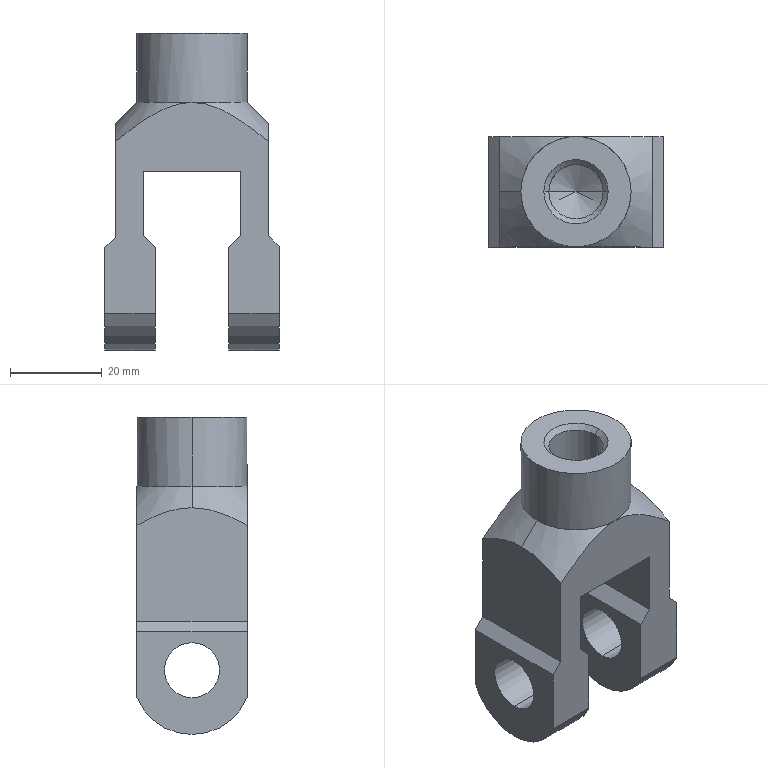Part | STEP file | Y_040B_Y-040B | 1 solid | 35 faces | box 38 x 24 x 69 mm | volume 28298 mm3 | plane 16 | cylinder 12 | cone 7 | commonest cylinder face diameters 12 x4 26 x4 11.84 x2 24 x2
STEP:
#1=CARTESIAN_POINT('',(0.,0.,-26.418));
#2=VERTEX_POINT('',#1);
#3=CARTESIAN_POINT('',(5.92,0.,-23.));
#4=VERTEX_POINT('',#3);
#5=CARTESIAN_POINT('',(0.,0.,-26.418));
#6=DIRECTION('',(0.866,0.,0.5));
#7=VECTOR('',#6,1000.);
#8=LINE('',#5,#7);
#9=EDGE_CURVE('',#2,#4,#8,.T.);
#10=ORIENTED_EDGE('',*,*,#9,.F.);
#11=CARTESIAN_POINT('',(-5.92,0.,-23.));
#12=VERTEX_POINT('',#11);
#13=CARTESIAN_POINT('',(0.,0.,-26.418));
#14=DIRECTION('',(-0.866,0.,0.5));
#15=VECTOR('',#14,1000.);
#16=LINE('',#13,#15);
#17=EDGE_CURVE('',#2,#12,#16,.T.);
#18=ORIENTED_EDGE('',*,*,#17,.T.);
#19=CARTESIAN_POINT('',(0.,0.,-23.));
#20=DIRECTION('',(0.,0.,1.));
#21=DIRECTION('',(1.,0.,0.));
#22=AXIS2_PLACEMENT_3D('',#19,#20,#21);
#23=CIRCLE('',#22,5.92);
#24=EDGE_CURVE('',#12,#4,#23,.T.);
#25=ORIENTED_EDGE('',*,*,#24,.T.);
#26=EDGE_LOOP('',(#10,#18,#25));
#27=FACE_OUTER_BOUND('',#26,.T.);
#28=CARTESIAN_POINT('',(0.,0.,973.582));
#29=DIRECTION('',(0.,0.,1.));
#30=DIRECTION('',(1.,0.,0.));
#31=AXIS2_PLACEMENT_3D('',#28,#29,#30);
#32=CONICAL_SURFACE('',#31,1732.051,1.047);
#33=ADVANCED_FACE('',(#27),#32,.F.);
#34=ORIENTED_EDGE('',*,*,#24,.F.);
#35=CARTESIAN_POINT('',(-5.92,0.,-1.08));
#36=VERTEX_POINT('',#35);
#37=CARTESIAN_POINT('',(-5.92,0.,-26.418));
#38=DIRECTION('',(0.,0.,1.));
#39=VECTOR('',#38,1000.);
#40=LINE('',#37,#39);
#41=EDGE_CURVE('',#12,#36,#40,.T.);
#42=ORIENTED_EDGE('',*,*,#41,.T.);
#43=CARTESIAN_POINT('',(5.92,0.,-1.08));
#44=VERTEX_POINT('',#43);
#45=CARTESIAN_POINT('',(0.,0.,-1.08));
#46=DIRECTION('',(0.,0.,1.));
#47=DIRECTION('',(1.,0.,0.));
#48=AXIS2_PLACEMENT_3D('',#45,#46,#47);
#49=CIRCLE('',#48,5.92);
#50=EDGE_CURVE('',#36,#44,#49,.T.);
#51=ORIENTED_EDGE('',*,*,#50,.T.);
#52=CARTESIAN_POINT('',(5.92,0.,-26.418));
#53=DIRECTION('',(0.,0.,1.));
#54=VECTOR('',#53,1000.);
#55=LINE('',#52,#54);
#56=EDGE_CURVE('',#4,#44,#55,.T.);
#57=ORIENTED_EDGE('',*,*,#56,.F.);
#58=EDGE_LOOP('',(#34,#42,#51,#57));
#59=FACE_OUTER_BOUND('',#58,.T.);
#60=CARTESIAN_POINT('',(0.,0.,-26.418));
#61=DIRECTION('',(0.,0.,1.));
#62=DIRECTION('',(1.,0.,0.));
#63=AXIS2_PLACEMENT_3D('',#60,#61,#62);
#64=CYLINDRICAL_SURFACE('',#63,5.92);
#65=ADVANCED_FACE('',(#59),#64,.F.);
#66=ORIENTED_EDGE('',*,*,#50,.F.);
#67=CARTESIAN_POINT('',(-7.,0.,0.));
#68=VERTEX_POINT('',#67);
#69=CARTESIAN_POINT('',(-5.92,0.,-1.08));
#70=DIRECTION('',(-0.7071,0.,0.7071));
#71=VECTOR('',#70,1000.);
#72=LINE('',#69,#71);
#73=EDGE_CURVE('',#36,#68,#72,.T.);
#74=ORIENTED_EDGE('',*,*,#73,.T.);
#75=CARTESIAN_POINT('',(7.,0.,0.));
#76=VERTEX_POINT('',#75);
#77=CARTESIAN_POINT('',(0.,0.,0.));
#78=DIRECTION('',(0.,0.,1.));
#79=DIRECTION('',(-1.,0.,0.));
#80=AXIS2_PLACEMENT_3D('',#77,#78,#79);
#81=CIRCLE('',#80,7.);
#82=EDGE_CURVE('',#68,#76,#81,.T.);
#83=ORIENTED_EDGE('',*,*,#82,.T.);
#84=CARTESIAN_POINT('',(5.92,0.,-1.08));
#85=DIRECTION('',(0.7071,0.,0.7071));
#86=VECTOR('',#85,1000.);
#87=LINE('',#84,#86);
#88=EDGE_CURVE('',#44,#76,#87,.T.);
#89=ORIENTED_EDGE('',*,*,#88,.F.);
#90=EDGE_LOOP('',(#66,#74,#83,#89));
#91=FACE_OUTER_BOUND('',#90,.T.);
#92=CARTESIAN_POINT('',(0.,0.,-1.08));
#93=DIRECTION('',(0.,0.,1.));
#94=DIRECTION('',(1.,0.,0.));
#95=AXIS2_PLACEMENT_3D('',#92,#93,#94);
#96=CONICAL_SURFACE('',#95,5.92,0.7854);
#97=ADVANCED_FACE('',(#91),#96,.F.);
#98=CARTESIAN_POINT('',(8.,0.,-49.));
#99=VERTEX_POINT('',#98);
#100=CARTESIAN_POINT('',(8.,0.,-61.));
#101=VERTEX_POINT('',#100);
#102=CARTESIAN_POINT('',(8.,0.,-55.));
#103=DIRECTION('',(1.,0.,0.));
#104=DIRECTION('',(0.,0.,-1.));
#105=AXIS2_PLACEMENT_3D('',#102,#103,#104);
#106=CIRCLE('',#105,6.);
#107=EDGE_CURVE('',#99,#101,#106,.T.);
#108=ORIENTED_EDGE('',*,*,#107,.F.);
#109=CARTESIAN_POINT('',(19.,0.,-49.));
#110=VERTEX_POINT('',#109);
#111=CARTESIAN_POINT('',(-24.,0.,-49.));
#112=DIRECTION('',(1.,0.,0.));
#113=VECTOR('',#112,1000.);
#114=LINE('',#111,#113);
#115=EDGE_CURVE('',#99,#110,#114,.T.);
#116=ORIENTED_EDGE('',*,*,#115,.T.);
#117=CARTESIAN_POINT('',(19.,0.,-61.));
#118=VERTEX_POINT('',#117);
#119=CARTESIAN_POINT('',(19.,0.,-55.));
#120=DIRECTION('',(-1.,0.,0.));
#121=DIRECTION('',(0.,0.,1.));
#122=AXIS2_PLACEMENT_3D('',#119,#120,#121);
#123=CIRCLE('',#122,6.);
#124=EDGE_CURVE('',#118,#110,#123,.T.);
#125=ORIENTED_EDGE('',*,*,#124,.F.);
#126=CARTESIAN_POINT('',(-24.,0.,-61.));
#127=DIRECTION('',(1.,0.,0.));
#128=VECTOR('',#127,1000.);
#129=LINE('',#126,#128);
#130=EDGE_CURVE('',#101,#118,#129,.T.);
#131=ORIENTED_EDGE('',*,*,#130,.F.);
#132=EDGE_LOOP('',(#108,#116,#125,#131));
#133=FACE_OUTER_BOUND('',#132,.T.);
#134=CARTESIAN_POINT('',(-24.,0.,-55.));
#135=DIRECTION('',(1.,0.,0.));
#136=DIRECTION('',(0.,0.,-1.));
#137=AXIS2_PLACEMENT_3D('',#134,#135,#136);
#138=CYLINDRICAL_SURFACE('',#137,6.);
#139=ADVANCED_FACE('',(#133),#138,.F.);
#140=CARTESIAN_POINT('',(-19.,0.,-49.));
#141=VERTEX_POINT('',#140);
#142=CARTESIAN_POINT('',(-19.,0.,-61.));
#143=VERTEX_POINT('',#142);
#144=CARTESIAN_POINT('',(-19.,0.,-55.));
#145=DIRECTION('',(1.,0.,0.));
#146=DIRECTION('',(0.,0.,-1.));
#147=AXIS2_PLACEMENT_3D('',#144,#145,#146);
#148=CIRCLE('',#147,6.);
#149=EDGE_CURVE('',#141,#143,#148,.T.);
#150=ORIENTED_EDGE('',*,*,#149,.F.);
#151=CARTESIAN_POINT('',(-8.,0.,-49.));
#152=VERTEX_POINT('',#151);
#153=CARTESIAN_POINT('',(-24.,0.,-49.));
#154=DIRECTION('',(1.,0.,0.));
#155=VECTOR('',#154,1000.);
#156=LINE('',#153,#155);
#157=EDGE_CURVE('',#141,#152,#156,.T.);
#158=ORIENTED_EDGE('',*,*,#157,.T.);
#159=CARTESIAN_POINT('',(-8.,0.,-61.));
#160=VERTEX_POINT('',#159);
#161=CARTESIAN_POINT('',(-8.,0.,-55.));
#162=DIRECTION('',(-1.,0.,0.));
#163=DIRECTION('',(0.,0.,1.));
#164=AXIS2_PLACEMENT_3D('',#161,#162,#163);
#165=CIRCLE('',#164,6.);
#166=EDGE_CURVE('',#160,#152,#165,.T.);
#167=ORIENTED_EDGE('',*,*,#166,.F.);
#168=CARTESIAN_POINT('',(-24.,0.,-61.));
#169=DIRECTION('',(1.,0.,0.));
#170=VECTOR('',#169,1000.);
#171=LINE('',#168,#170);
#172=EDGE_CURVE('',#143,#160,#171,.T.);
#173=ORIENTED_EDGE('',*,*,#172,.F.);
#174=EDGE_LOOP('',(#150,#158,#167,#173));
#175=FACE_OUTER_BOUND('',#174,.T.);
#176=CARTESIAN_POINT('',(-24.,0.,-55.));
#177=DIRECTION('',(1.,0.,0.));
#178=DIRECTION('',(0.,0.,-1.));
#179=AXIS2_PLACEMENT_3D('',#176,#177,#178);
#180=CYLINDRICAL_SURFACE('',#179,6.);
#181=ADVANCED_FACE('',(#175),#180,.F.);
#182=CARTESIAN_POINT('',(8.,0.,-69.));
#183=VERTEX_POINT('',#182);
#184=CARTESIAN_POINT('',(8.,-12.,-61.));
#185=VERTEX_POINT('',#184);
#186=CARTESIAN_POINT('',(8.,0.,-56.));
#187=DIRECTION('',(-1.,0.,0.));
#188=DIRECTION('',(0.,0.,-1.));
#189=AXIS2_PLACEMENT_3D('',#186,#187,#188);
#190=CIRCLE('',#189,13.);
#191=EDGE_CURVE('',#183,#185,#190,.T.);
#192=ORIENTED_EDGE('',*,*,#191,.F.);
#193=CARTESIAN_POINT('',(19.,0.,-69.));
#194=VERTEX_POINT('',#193);
#195=CARTESIAN_POINT('',(-24.,0.,-69.));
#196=DIRECTION('',(1.,0.,0.));
#197=VECTOR('',#196,1000.);
#198=LINE('',#195,#197);
#199=EDGE_CURVE('',#183,#194,#198,.T.);
#200=ORIENTED_EDGE('',*,*,#199,.T.);
#201=CARTESIAN_POINT('',(19.,-12.,-61.));
#202=VERTEX_POINT('',#201);
#203=CARTESIAN_POINT('',(19.,0.,-56.));
#204=DIRECTION('',(1.,0.,0.));
#205=DIRECTION('',(0.,0.,1.));
#206=AXIS2_PLACEMENT_3D('',#203,#204,#205);
#207=CIRCLE('',#206,13.);
#208=EDGE_CURVE('',#202,#194,#207,.T.);
#209=ORIENTED_EDGE('',*,*,#208,.F.);
#210=CARTESIAN_POINT('',(-24.,-12.,-61.));
#211=DIRECTION('',(1.,0.,0.));
#212=VECTOR('',#211,1000.);
#213=LINE('',#210,#212);
#214=EDGE_CURVE('',#185,#202,#213,.T.);
#215=ORIENTED_EDGE('',*,*,#214,.F.);
#216=EDGE_LOOP('',(#192,#200,#209,#215));
#217=FACE_OUTER_BOUND('',#216,.T.);
#218=CARTESIAN_POINT('',(-24.,0.,-56.));
#219=DIRECTION('',(1.,0.,0.));
#220=DIRECTION('',(0.,0.,-1.));
#221=AXIS2_PLACEMENT_3D('',#218,#219,#220);
#222=CYLINDRICAL_SURFACE('',#221,13.);
#223=ADVANCED_FACE('',(#217),#222,.T.);
#224=CARTESIAN_POINT('',(-19.,0.,-69.));
#225=VERTEX_POINT('',#224);
#226=CARTESIAN_POINT('',(-19.,-12.,-61.));
#227=VERTEX_POINT('',#226);
#228=CARTESIAN_POINT('',(-19.,0.,-56.));
#229=DIRECTION('',(-1.,0.,0.));
#230=DIRECTION('',(0.,0.,-1.));
#231=AXIS2_PLACEMENT_3D('',#228,#229,#230);
#232=CIRCLE('',#231,13.);
#233=EDGE_CURVE('',#225,#227,#232,.T.);
#234=ORIENTED_EDGE('',*,*,#233,.F.);
#235=CARTESIAN_POINT('',(-8.,0.,-69.));
#236=VERTEX_POINT('',#235);
#237=CARTESIAN_POINT('',(-24.,0.,-69.));
#238=DIRECTION('',(1.,0.,0.));
#239=VECTOR('',#238,1000.);
#240=LINE('',#237,#239);
#241=EDGE_CURVE('',#225,#236,#240,.T.);
#242=ORIENTED_EDGE('',*,*,#241,.T.);
#243=CARTESIAN_POINT('',(-8.,-12.,-61.));
#244=VERTEX_POINT('',#243);
#245=CARTESIAN_POINT('',(-8.,0.,-56.));
#246=DIRECTION('',(1.,0.,0.));
#247=DIRECTION('',(0.,0.,1.));
#248=AXIS2_PLACEMENT_3D('',#245,#246,#247);
#249=CIRCLE('',#248,13.);
#250=EDGE_CURVE('',#244,#236,#249,.T.);
#251=ORIENTED_EDGE('',*,*,#250,.F.);
#252=CARTESIAN_POINT('',(-24.,-12.,-61.));
#253=DIRECTION('',(1.,0.,0.));
#254=VECTOR('',#253,1000.);
#255=LINE('',#252,#254);
#256=EDGE_CURVE('',#227,#244,#255,.T.);
#257=ORIENTED_EDGE('',*,*,#256,.F.);
#258=EDGE_LOOP('',(#234,#242,#251,#257));
#259=FACE_OUTER_BOUND('',#258,.T.);
#260=CARTESIAN_POINT('',(-24.,0.,-56.));
#261=DIRECTION('',(1.,0.,0.));
#262=DIRECTION('',(0.,0.,-1.));
#263=AXIS2_PLACEMENT_3D('',#260,#261,#262);
#264=CYLINDRICAL_SURFACE('',#263,13.);
#265=ADVANCED_FACE('',(#259),#264,.T.);
#266=CARTESIAN_POINT('',(0.,12.,-15.));
#267=VERTEX_POINT('',#266);
#268=CARTESIAN_POINT('',(-12.,0.,-15.));
#269=VERTEX_POINT('',#268);
#270=CARTESIAN_POINT('',(0.,0.,-15.));
#271=DIRECTION('',(0.,0.,1.));
#272=DIRECTION('',(1.,0.,0.));
#273=AXIS2_PLACEMENT_3D('',#270,#271,#272);
#274=CIRCLE('',#273,12.);
#275=EDGE_CURVE('',#267,#269,#274,.T.);
#276=ORIENTED_EDGE('',*,*,#275,.T.);
#277=CARTESIAN_POINT('',(-12.,0.,0.));
#278=VERTEX_POINT('',#277);
#279=CARTESIAN_POINT('',(-12.,0.,-30.));
#280=DIRECTION('',(0.,0.,1.));
#281=VECTOR('',#280,1000.);
#282=LINE('',#279,#281);
#283=EDGE_CURVE('',#269,#278,#282,.T.);
#284=ORIENTED_EDGE('',*,*,#283,.T.);
#285=CARTESIAN_POINT('',(12.,0.,0.));
#286=VERTEX_POINT('',#285);
#287=CARTESIAN_POINT('',(0.,0.,0.));
#288=DIRECTION('',(0.,0.,1.));
#289=DIRECTION('',(1.,0.,0.));
#290=AXIS2_PLACEMENT_3D('',#287,#288,#289);
#291=CIRCLE('',#290,12.);
#292=EDGE_CURVE('',#286,#278,#291,.T.);
#293=ORIENTED_EDGE('',*,*,#292,.F.);
#294=CARTESIAN_POINT('',(12.,0.,-15.));
#295=VERTEX_POINT('',#294);
#296=CARTESIAN_POINT('',(12.,0.,-30.));
#297=DIRECTION('',(0.,0.,1.));
#298=VECTOR('',#297,1000.);
#299=LINE('',#296,#298);
#300=EDGE_CURVE('',#295,#286,#299,.T.);
#301=ORIENTED_EDGE('',*,*,#300,.F.);
#302=CARTESIAN_POINT('',(0.,0.,-15.));
#303=DIRECTION('',(0.,0.,1.));
#304=DIRECTION('',(1.,0.,0.));
#305=AXIS2_PLACEMENT_3D('',#302,#303,#304);
#306=CIRCLE('',#305,12.);
#307=EDGE_CURVE('',#295,#267,#306,.T.);
#308=ORIENTED_EDGE('',*,*,#307,.T.);
#309=EDGE_LOOP('',(#276,#284,#293,#301,#308));
#310=FACE_OUTER_BOUND('',#309,.T.);
#311=CARTESIAN_POINT('',(0.,0.,-30.));
#312=DIRECTION('',(0.,0.,1.));
#313=DIRECTION('',(1.,0.,0.));
#314=AXIS2_PLACEMENT_3D('',#311,#312,#313);
#315=CYLINDRICAL_SURFACE('',#314,12.);
#316=ADVANCED_FACE('',(#310),#315,.T.);
#317=CARTESIAN_POINT('',(0.,-12.,-15.));
#318=VERTEX_POINT('',#317);
#319=CARTESIAN_POINT('',(0.,0.,-15.));
#320=DIRECTION('',(0.,0.,1.));
#321=DIRECTION('',(1.,0.,0.));
#322=AXIS2_PLACEMENT_3D('',#319,#320,#321);
#323=CIRCLE('',#322,12.);
#324=EDGE_CURVE('',#269,#318,#323,.T.);
#325=ORIENTED_EDGE('',*,*,#324,.F.);
#326=CARTESIAN_POINT('',(-16.65,0.,-19.65));
#327=VERTEX_POINT('',#326);
#328=CARTESIAN_POINT('',(-16.65,0.,-19.65));
#329=DIRECTION('',(-0.7071,0.,-0.7071));
#330=VECTOR('',#329,1000.);
#331=LINE('',#328,#330);
#332=EDGE_CURVE('',#269,#327,#331,.T.);
#333=ORIENTED_EDGE('',*,*,#332,.T.);
#334=CARTESIAN_POINT('',(-16.65,-12.,-23.524));
#335=VERTEX_POINT('',#334);
#336=CARTESIAN_POINT('',(-16.65,0.,-19.65));
#337=CARTESIAN_POINT('',(-16.65,-0.5346,-19.65));
#338=CARTESIAN_POINT('',(-16.65,-1.075,-19.676));
#339=CARTESIAN_POINT('',(-16.65,-2.146,-19.779));
#340=CARTESIAN_POINT('',(-16.65,-2.674,-19.856));
#341=CARTESIAN_POINT('',(-16.65,-4.237,-20.15));
#342=CARTESIAN_POINT('',(-16.65,-5.253,-20.434));
#343=CARTESIAN_POINT('',(-16.65,-7.245,-21.134));
#344=CARTESIAN_POINT('',(-16.65,-8.221,-21.55));
#345=CARTESIAN_POINT('',(-16.65,-9.663,-22.246));
#346=CARTESIAN_POINT('',(-16.65,-10.14,-22.49));
#347=CARTESIAN_POINT('',(-16.65,-11.078,-22.995));
#348=CARTESIAN_POINT('',(-16.65,-11.542,-23.256));
#349=CARTESIAN_POINT('',(-16.65,-12.,-23.524));
#350=B_SPLINE_CURVE_WITH_KNOTS('',3,(#336,#337,#338,#339,#340,#341,#342,#343,#344,#345,#346,#347,#348,#349),.UNSPECIFIED.,.F.,.F.,(4,2,2,2,2,2,4),(0.06464,0.06623,0.06782,0.071,0.07418,0.07576,0.07735),.UNSPECIFIED.);
#351=EDGE_CURVE('',#327,#335,#350,.T.);
#352=ORIENTED_EDGE('',*,*,#351,.T.);
#353=CARTESIAN_POINT('',(-16.65,-12.,-23.524));
#354=CARTESIAN_POINT('',(-15.42,-12.,-22.526));
#355=CARTESIAN_POINT('',(-14.172,-12.,-21.55));
#356=CARTESIAN_POINT('',(-12.254,-12.,-20.145));
#357=CARTESIAN_POINT('',(-11.606,-12.,-19.687));
#358=CARTESIAN_POINT('',(-10.288,-12.,-18.799));
#359=CARTESIAN_POINT('',(-9.617,-12.,-18.368));
#360=CARTESIAN_POINT('',(-8.251,-12.,-17.553));
#361=CARTESIAN_POINT('',(-7.558,-12.,-17.168));
#362=CARTESIAN_POINT('',(-6.139,-12.,-16.465));
#363=CARTESIAN_POINT('',(-5.414,-12.,-16.146));
#364=CARTESIAN_POINT('',(-3.919,-12.,-15.604));
#365=CARTESIAN_POINT('',(-3.143,-12.,-15.381));
#366=CARTESIAN_POINT('',(-1.585,-12.,-15.08));
#367=CARTESIAN_POINT('',(-0.7974,-12.,-15.));
#368=CARTESIAN_POINT('',(0.,-12.,-15.));
#369=B_SPLINE_CURVE_WITH_KNOTS('',3,(#353,#354,#355,#356,#357,#358,#359,#360,#361,#362,#363,#364,#365,#366,#367,#368),.UNSPECIFIED.,.F.,.F.,(4,2,2,2,2,2,2,4),(0.009557,0.01431,0.01668,0.01906,0.02144,0.02381,0.02619,0.02856),.UNSPECIFIED.);
#370=EDGE_CURVE('',#335,#318,#369,.T.);
#371=ORIENTED_EDGE('',*,*,#370,.T.);
#372=EDGE_LOOP('',(#325,#333,#352,#371));
#373=FACE_OUTER_BOUND('',#372,.T.);
#374=CARTESIAN_POINT('',(0.,0.,-19.65));
#375=DIRECTION('',(0.,0.,-1.));
#376=DIRECTION('',(-1.,0.,0.));
#377=AXIS2_PLACEMENT_3D('',#374,#375,#376);
#378=CONICAL_SURFACE('',#377,16.65,0.7854);
#379=ADVANCED_FACE('',(#373),#378,.T.);
#380=ORIENTED_EDGE('',*,*,#292,.T.);
#381=CARTESIAN_POINT('',(0.,0.,0.));
#382=DIRECTION('',(0.,0.,1.));
#383=DIRECTION('',(1.,0.,0.));
#384=AXIS2_PLACEMENT_3D('',#381,#382,#383);
#385=CIRCLE('',#384,12.);
#386=EDGE_CURVE('',#278,#286,#385,.T.);
#387=ORIENTED_EDGE('',*,*,#386,.T.);
#388=EDGE_LOOP('',(#380,#387));
#389=FACE_OUTER_BOUND('',#388,.T.);
#390=CARTESIAN_POINT('',(0.,0.,0.));
#391=DIRECTION('',(0.,0.,1.));
#392=DIRECTION('',(-1.,0.,0.));
#393=AXIS2_PLACEMENT_3D('',#390,#391,#392);
#394=CIRCLE('',#393,7.);
#395=EDGE_CURVE('',#76,#68,#394,.T.);
#396=ORIENTED_EDGE('',*,*,#395,.F.);
#397=ORIENTED_EDGE('',*,*,#82,.F.);
#398=EDGE_LOOP('',(#396,#397));
#399=FACE_BOUND('',#398,.T.);
#400=CARTESIAN_POINT('',(0.,0.,0.));
#401=DIRECTION('',(0.,0.,-1.));
#402=DIRECTION('',(-1.,0.,0.));
#403=AXIS2_PLACEMENT_3D('',#400,#401,#402);
#404=PLANE('',#403);
#405=ADVANCED_FACE('',(#389,#399),#404,.F.);
#406=CARTESIAN_POINT('',(-19.,12.,-61.));
#407=VERTEX_POINT('',#406);
#408=CARTESIAN_POINT('',(-8.,12.,-61.));
#409=VERTEX_POINT('',#408);
#410=CARTESIAN_POINT('',(-24.,12.,-61.));
#411=DIRECTION('',(1.,0.,0.));
#412=VECTOR('',#411,1000.);
#413=LINE('',#410,#412);
#414=EDGE_CURVE('',#407,#409,#413,.T.);
#415=ORIENTED_EDGE('',*,*,#414,.F.);
#416=CARTESIAN_POINT('',(-19.,12.,-46.65));
#417=VERTEX_POINT('',#416);
#418=CARTESIAN_POINT('',(-19.,12.,-69.));
#419=DIRECTION('',(0.,0.,1.));
#420=VECTOR('',#419,1000.);
#421=LINE('',#418,#420);
#422=EDGE_CURVE('',#407,#417,#421,.T.);
#423=ORIENTED_EDGE('',*,*,#422,.T.);
#424=CARTESIAN_POINT('',(-16.65,12.,-44.3));
#425=VERTEX_POINT('',#424);
#426=CARTESIAN_POINT('',(-19.,12.,-46.65));
#427=DIRECTION('',(0.7071,0.,0.7071));
#428=VECTOR('',#427,1000.);
#429=LINE('',#426,#428);
#430=EDGE_CURVE('',#417,#425,#429,.T.);
#431=ORIENTED_EDGE('',*,*,#430,.T.);
#432=CARTESIAN_POINT('',(-16.65,12.,-23.524));
#433=VERTEX_POINT('',#432);
#434=CARTESIAN_POINT('',(-16.65,12.,-44.3));
#435=DIRECTION('',(0.,0.,1.));
#436=VECTOR('',#435,1000.);
#437=LINE('',#434,#436);
#438=EDGE_CURVE('',#425,#433,#437,.T.);
#439=ORIENTED_EDGE('',*,*,#438,.T.);
#440=CARTESIAN_POINT('',(-16.65,12.,-23.524));
#441=CARTESIAN_POINT('',(-15.42,12.,-22.526));
#442=CARTESIAN_POINT('',(-14.172,12.,-21.55));
#443=CARTESIAN_POINT('',(-12.254,12.,-20.145));
#444=CARTESIAN_POINT('',(-11.606,12.,-19.687));
#445=CARTESIAN_POINT('',(-10.288,12.,-18.799));
#446=CARTESIAN_POINT('',(-9.617,12.,-18.368));
#447=CARTESIAN_POINT('',(-8.251,12.,-17.553));
#448=CARTESIAN_POINT('',(-7.558,12.,-17.168));
#449=CARTESIAN_POINT('',(-6.139,12.,-16.465));
#450=CARTESIAN_POINT('',(-5.414,12.,-16.146));
#451=CARTESIAN_POINT('',(-3.919,12.,-15.604));
#452=CARTESIAN_POINT('',(-3.143,12.,-15.381));
#453=CARTESIAN_POINT('',(-1.585,12.,-15.08));
#454=CARTESIAN_POINT('',(-0.7974,12.,-15.));
#455=CARTESIAN_POINT('',(0.,12.,-15.));
#456=B_SPLINE_CURVE_WITH_KNOTS('',3,(#440,#441,#442,#443,#444,#445,#446,#447,#448,#449,#450,#451,#452,#453,#454,#455),.UNSPECIFIED.,.F.,.F.,(4,2,2,2,2,2,2,4),(0.009557,0.01431,0.01668,0.01906,0.02144,0.02381,0.02619,0.02856),.UNSPECIFIED.);
#457=EDGE_CURVE('',#433,#267,#456,.T.);
#458=ORIENTED_EDGE('',*,*,#457,.T.);
#459=CARTESIAN_POINT('',(16.65,12.,-23.524));
#460=VERTEX_POINT('',#459);
#461=CARTESIAN_POINT('',(0.,12.,-15.));
#462=CARTESIAN_POINT('',(0.3995,12.,-15.));
#463=CARTESIAN_POINT('',(0.8034,12.,-15.02));
#464=CARTESIAN_POINT('',(1.6,12.,-15.1));
#465=CARTESIAN_POINT('',(1.994,12.,-15.159));
#466=CARTESIAN_POINT('',(3.165,12.,-15.387));
#467=CARTESIAN_POINT('',(3.93,12.,-15.607));
#468=CARTESIAN_POINT('',(5.059,12.,-16.018));
#469=CARTESIAN_POINT('',(5.432,12.,-16.168));
#470=CARTESIAN_POINT('',(6.162,12.,-16.486));
#471=CARTESIAN_POINT('',(6.522,12.,-16.654));
#472=CARTESIAN_POINT('',(7.585,12.,-17.183));
#473=CARTESIAN_POINT('',(8.276,12.,-17.567));
#474=CARTESIAN_POINT('',(10.308,12.,-18.782));
#475=CARTESIAN_POINT('',(11.611,12.,-19.675));
#476=CARTESIAN_POINT('',(14.168,12.,-21.546));
#477=CARTESIAN_POINT('',(15.42,12.,-22.526));
#478=CARTESIAN_POINT('',(16.65,12.,-23.524));
#479=B_SPLINE_CURVE_WITH_KNOTS('',3,(#461,#462,#463,#464,#465,#466,#467,#468,#469,#470,#471,#472,#473,#474,#475,#476,#477,#478),.UNSPECIFIED.,.F.,.F.,(4,2,2,2,2,2,2,2,4),(0.02856,0.02975,0.03094,0.03333,0.03452,0.03571,0.03809,0.04285,0.04761),.UNSPECIFIED.);
#480=EDGE_CURVE('',#267,#460,#479,.T.);
#481=ORIENTED_EDGE('',*,*,#480,.T.);
#482=CARTESIAN_POINT('',(16.65,12.,-44.));
#483=VERTEX_POINT('',#482);
#484=CARTESIAN_POINT('',(16.65,12.,-19.6));
#485=DIRECTION('',(0.,0.,-1.));
#486=VECTOR('',#485,1000.);
#487=LINE('',#484,#486);
#488=EDGE_CURVE('',#460,#483,#487,.T.);
#489=ORIENTED_EDGE('',*,*,#488,.T.);
#490=CARTESIAN_POINT('',(19.,12.,-46.35));
#491=VERTEX_POINT('',#490);
#492=CARTESIAN_POINT('',(16.65,12.,-44.));
#493=DIRECTION('',(0.7071,0.,-0.7071));
#494=VECTOR('',#493,1000.);
#495=LINE('',#492,#494);
#496=EDGE_CURVE('',#483,#491,#495,.T.);
#497=ORIENTED_EDGE('',*,*,#496,.T.);
#498=CARTESIAN_POINT('',(19.,12.,-61.));
#499=VERTEX_POINT('',#498);
#500=CARTESIAN_POINT('',(19.,12.,-46.35));
#501=DIRECTION('',(0.,0.,-1.));
#502=VECTOR('',#501,1000.);
#503=LINE('',#500,#502);
#504=EDGE_CURVE('',#491,#499,#503,.T.);
#505=ORIENTED_EDGE('',*,*,#504,.T.);
#506=CARTESIAN_POINT('',(8.,12.,-61.));
#507=VERTEX_POINT('',#506);
#508=CARTESIAN_POINT('',(-24.,12.,-61.));
#509=DIRECTION('',(1.,0.,0.));
#510=VECTOR('',#509,1000.);
#511=LINE('',#508,#510);
#512=EDGE_CURVE('',#507,#499,#511,.T.);
#513=ORIENTED_EDGE('',*,*,#512,.F.);
#514=CARTESIAN_POINT('',(8.,12.,-46.65));
#515=VERTEX_POINT('',#514);
#516=CARTESIAN_POINT('',(8.,12.,-69.));
#517=DIRECTION('',(0.,0.,1.));
#518=VECTOR('',#517,1000.);
#519=LINE('',#516,#518);
#520=EDGE_CURVE('',#507,#515,#519,.T.);
#521=ORIENTED_EDGE('',*,*,#520,.T.);
#522=CARTESIAN_POINT('',(10.65,12.,-44.));
#523=VERTEX_POINT('',#522);
#524=CARTESIAN_POINT('',(8.,12.,-46.65));
#525=DIRECTION('',(0.7071,0.,0.7071));
#526=VECTOR('',#525,1000.);
#527=LINE('',#524,#526);
#528=EDGE_CURVE('',#515,#523,#527,.T.);
#529=ORIENTED_EDGE('',*,*,#528,.T.);
#530=CARTESIAN_POINT('',(10.65,12.,-30.));
#531=VERTEX_POINT('',#530);
#532=CARTESIAN_POINT('',(10.65,12.,-44.));
#533=DIRECTION('',(0.,0.,1.));
#534=VECTOR('',#533,1000.);
#535=LINE('',#532,#534);
#536=EDGE_CURVE('',#523,#531,#535,.T.);
#537=ORIENTED_EDGE('',*,*,#536,.T.);
#538=CARTESIAN_POINT('',(-10.65,12.,-30.));
#539=VERTEX_POINT('',#538);
#540=CARTESIAN_POINT('',(10.65,12.,-30.));
#541=DIRECTION('',(-1.,0.,0.));
#542=VECTOR('',#541,1000.);
#543=LINE('',#540,#542);
#544=EDGE_CURVE('',#531,#539,#543,.T.);
#545=ORIENTED_EDGE('',*,*,#544,.T.);
#546=CARTESIAN_POINT('',(-10.65,12.,-44.));
#547=VERTEX_POINT('',#546);
#548=CARTESIAN_POINT('',(-10.65,12.,-30.));
#549=DIRECTION('',(0.,0.,-1.));
#550=VECTOR('',#549,1000.);
#551=LINE('',#548,#550);
#552=EDGE_CURVE('',#539,#547,#551,.T.);
#553=ORIENTED_EDGE('',*,*,#552,.T.);
#554=CARTESIAN_POINT('',(-8.,12.,-46.65));
#555=VERTEX_POINT('',#554);
#556=CARTESIAN_POINT('',(-10.65,12.,-44.));
#557=DIRECTION('',(0.7071,0.,-0.7071));
#558=VECTOR('',#557,1000.);
#559=LINE('',#556,#558);
#560=EDGE_CURVE('',#547,#555,#559,.T.);
#561=ORIENTED_EDGE('',*,*,#560,.T.);
#562=CARTESIAN_POINT('',(-8.,12.,-46.65));
#563=DIRECTION('',(0.,0.,-1.));
#564=VECTOR('',#563,1000.);
#565=LINE('',#562,#564);
#566=EDGE_CURVE('',#555,#409,#565,.T.);
#567=ORIENTED_EDGE('',*,*,#566,.T.);
#568=EDGE_LOOP('',(#415,#423,#431,#439,#458,#481,#489,#497,#505,#513,#521,#529,#537,#545,#553,#561,#567));
#569=FACE_OUTER_BOUND('',#568,.T.);
#570=CARTESIAN_POINT('',(-20.,12.,-15.));
#571=DIRECTION('',(0.,1.,0.));
#572=DIRECTION('',(0.,0.,1.));
#573=AXIS2_PLACEMENT_3D('',#570,#571,#572);
#574=PLANE('',#573);
#575=ADVANCED_FACE('',(#569),#574,.T.);
#576=CARTESIAN_POINT('',(-19.,-12.,-46.65));
#577=VERTEX_POINT('',#576);
#578=CARTESIAN_POINT('',(-19.,-12.,-69.));
#579=DIRECTION('',(0.,0.,1.));
#580=VECTOR('',#579,1000.);
#581=LINE('',#578,#580);
#582=EDGE_CURVE('',#227,#577,#581,.T.);
#583=ORIENTED_EDGE('',*,*,#582,.F.);
#584=ORIENTED_EDGE('',*,*,#256,.T.);
#585=CARTESIAN_POINT('',(-8.,-12.,-46.65));
#586=VERTEX_POINT('',#585);
#587=CARTESIAN_POINT('',(-8.,-12.,-46.65));
#588=DIRECTION('',(0.,0.,-1.));
#589=VECTOR('',#588,1000.);
#590=LINE('',#587,#589);
#591=EDGE_CURVE('',#586,#244,#590,.T.);
#592=ORIENTED_EDGE('',*,*,#591,.F.);
#593=CARTESIAN_POINT('',(-10.65,-12.,-44.));
#594=VERTEX_POINT('',#593);
#595=CARTESIAN_POINT('',(-10.65,-12.,-44.));
#596=DIRECTION('',(0.7071,0.,-0.7071));
#597=VECTOR('',#596,1000.);
#598=LINE('',#595,#597);
#599=EDGE_CURVE('',#594,#586,#598,.T.);
#600=ORIENTED_EDGE('',*,*,#599,.F.);
#601=CARTESIAN_POINT('',(-10.65,-12.,-30.));
#602=VERTEX_POINT('',#601);
#603=CARTESIAN_POINT('',(-10.65,-12.,-30.));
#604=DIRECTION('',(0.,0.,-1.));
#605=VECTOR('',#604,1000.);
#606=LINE('',#603,#605);
#607=EDGE_CURVE('',#602,#594,#606,.T.);
#608=ORIENTED_EDGE('',*,*,#607,.F.);
#609=CARTESIAN_POINT('',(10.65,-12.,-30.));
#610=VERTEX_POINT('',#609);
#611=CARTESIAN_POINT('',(10.65,-12.,-30.));
#612=DIRECTION('',(-1.,0.,0.));
#613=VECTOR('',#612,1000.);
#614=LINE('',#611,#613);
#615=EDGE_CURVE('',#610,#602,#614,.T.);
#616=ORIENTED_EDGE('',*,*,#615,.F.);
#617=CARTESIAN_POINT('',(10.65,-12.,-44.));
#618=VERTEX_POINT('',#617);
#619=CARTESIAN_POINT('',(10.65,-12.,-44.));
#620=DIRECTION('',(0.,0.,1.));
#621=VECTOR('',#620,1000.);
#622=LINE('',#619,#621);
#623=EDGE_CURVE('',#618,#610,#622,.T.);
#624=ORIENTED_EDGE('',*,*,#623,.F.);
#625=CARTESIAN_POINT('',(8.,-12.,-46.65));
#626=VERTEX_POINT('',#625);
#627=CARTESIAN_POINT('',(8.,-12.,-46.65));
#628=DIRECTION('',(0.7071,0.,0.7071));
#629=VECTOR('',#628,1000.);
#630=LINE('',#627,#629);
#631=EDGE_CURVE('',#626,#618,#630,.T.);
#632=ORIENTED_EDGE('',*,*,#631,.F.);
#633=CARTESIAN_POINT('',(8.,-12.,-69.));
#634=DIRECTION('',(0.,0.,1.));
#635=VECTOR('',#634,1000.);
#636=LINE('',#633,#635);
#637=EDGE_CURVE('',#185,#626,#636,.T.);
#638=ORIENTED_EDGE('',*,*,#637,.F.);
#639=ORIENTED_EDGE('',*,*,#214,.T.);
#640=CARTESIAN_POINT('',(19.,-12.,-46.35));
#641=VERTEX_POINT('',#640);
#642=CARTESIAN_POINT('',(19.,-12.,-46.35));
#643=DIRECTION('',(0.,0.,-1.));
#644=VECTOR('',#643,1000.);
#645=LINE('',#642,#644);
#646=EDGE_CURVE('',#641,#202,#645,.T.);
#647=ORIENTED_EDGE('',*,*,#646,.F.);
#648=CARTESIAN_POINT('',(16.65,-12.,-44.));
#649=VERTEX_POINT('',#648);
#650=CARTESIAN_POINT('',(16.65,-12.,-44.));
#651=DIRECTION('',(0.7071,0.,-0.7071));
#652=VECTOR('',#651,1000.);
#653=LINE('',#650,#652);
#654=EDGE_CURVE('',#649,#641,#653,.T.);
#655=ORIENTED_EDGE('',*,*,#654,.F.);
#656=CARTESIAN_POINT('',(16.65,-12.,-23.524));
#657=VERTEX_POINT('',#656);
#658=CARTESIAN_POINT('',(16.65,-12.,-19.6));
#659=DIRECTION('',(0.,0.,-1.));
#660=VECTOR('',#659,1000.);
#661=LINE('',#658,#660);
#662=EDGE_CURVE('',#657,#649,#661,.T.);
#663=ORIENTED_EDGE('',*,*,#662,.F.);
#664=CARTESIAN_POINT('',(0.,-12.,-15.));
#665=CARTESIAN_POINT('',(0.3995,-12.,-15.));
#666=CARTESIAN_POINT('',(0.8034,-12.,-15.02));
#667=CARTESIAN_POINT('',(1.6,-12.,-15.1));
#668=CARTESIAN_POINT('',(1.994,-12.,-15.159));
#669=CARTESIAN_POINT('',(3.165,-12.,-15.387));
#670=CARTESIAN_POINT('',(3.93,-12.,-15.607));
#671=CARTESIAN_POINT('',(5.059,-12.,-16.018));
#672=CARTESIAN_POINT('',(5.432,-12.,-16.168));
#673=CARTESIAN_POINT('',(6.162,-12.,-16.486));
#674=CARTESIAN_POINT('',(6.522,-12.,-16.654));
#675=CARTESIAN_POINT('',(7.585,-12.,-17.183));
#676=CARTESIAN_POINT('',(8.276,-12.,-17.567));
#677=CARTESIAN_POINT('',(10.308,-12.,-18.782));
#678=CARTESIAN_POINT('',(11.611,-12.,-19.675));
#679=CARTESIAN_POINT('',(14.168,-12.,-21.546));
#680=CARTESIAN_POINT('',(15.42,-12.,-22.526));
#681=CARTESIAN_POINT('',(16.65,-12.,-23.524));
#682=B_SPLINE_CURVE_WITH_KNOTS('',3,(#664,#665,#666,#667,#668,#669,#670,#671,#672,#673,#674,#675,#676,#677,#678,#679,#680,#681),.UNSPECIFIED.,.F.,.F.,(4,2,2,2,2,2,2,2,4),(0.02856,0.02975,0.03094,0.03333,0.03452,0.03571,0.03809,0.04285,0.04761),.UNSPECIFIED.);
#683=EDGE_CURVE('',#318,#657,#682,.T.);
#684=ORIENTED_EDGE('',*,*,#683,.F.);
#685=ORIENTED_EDGE('',*,*,#370,.F.);
#686=CARTESIAN_POINT('',(-16.65,-12.,-44.3));
#687=VERTEX_POINT('',#686);
#688=CARTESIAN_POINT('',(-16.65,-12.,-44.3));
#689=DIRECTION('',(0.,0.,1.));
#690=VECTOR('',#689,1000.);
#691=LINE('',#688,#690);
#692=EDGE_CURVE('',#687,#335,#691,.T.);
#693=ORIENTED_EDGE('',*,*,#692,.F.);
#694=CARTESIAN_POINT('',(-19.,-12.,-46.65));
#695=DIRECTION('',(0.7071,0.,0.7071));
#696=VECTOR('',#695,1000.);
#697=LINE('',#694,#696);
#698=EDGE_CURVE('',#577,#687,#697,.T.);
#699=ORIENTED_EDGE('',*,*,#698,.F.);
#700=EDGE_LOOP('',(#583,#584,#592,#600,#608,#616,#624,#632,#638,#639,#647,#655,#663,#684,#685,#693,#699));
#701=FACE_OUTER_BOUND('',#700,.T.);
#702=CARTESIAN_POINT('',(-20.,-12.,-15.));
#703=DIRECTION('',(0.,1.,0.));
#704=DIRECTION('',(0.,0.,1.));
#705=AXIS2_PLACEMENT_3D('',#702,#703,#704);
#706=PLANE('',#705);
#707=ADVANCED_FACE('',(#701),#706,.F.);
#708=CARTESIAN_POINT('',(-16.65,12.,-23.524));
#709=CARTESIAN_POINT('',(-16.65,11.082,-22.987));
#710=CARTESIAN_POINT('',(-16.65,10.149,-22.481));
#711=CARTESIAN_POINT('',(-16.65,8.24,-21.558));
#712=CARTESIAN_POINT('',(-16.65,7.264,-21.141));
#713=CARTESIAN_POINT('',(-16.65,5.755,-20.61));
#714=CARTESIAN_POINT('',(-16.65,5.243,-20.449));
#715=CARTESIAN_POINT('',(-16.65,4.208,-20.166));
#716=CARTESIAN_POINT('',(-16.65,3.688,-20.046));
#717=CARTESIAN_POINT('',(-16.65,2.121,-19.753));
#718=CARTESIAN_POINT('',(-16.65,1.066,-19.65));
#719=CARTESIAN_POINT('',(-16.65,0.,-19.65));
#720=B_SPLINE_CURVE_WITH_KNOTS('',3,(#708,#709,#710,#711,#712,#713,#714,#715,#716,#717,#718,#719),.UNSPECIFIED.,.F.,.F.,(4,2,2,2,2,4),(0.05197,0.05514,0.0583,0.05989,0.06147,0.06464),.UNSPECIFIED.);
#721=EDGE_CURVE('',#433,#327,#720,.T.);
#722=ORIENTED_EDGE('',*,*,#721,.F.);
#723=ORIENTED_EDGE('',*,*,#438,.F.);
#724=CARTESIAN_POINT('',(-16.65,12.,-44.3));
#725=DIRECTION('',(0.,-1.,0.));
#726=VECTOR('',#725,1000.);
#727=LINE('',#724,#726);
#728=EDGE_CURVE('',#425,#687,#727,.T.);
#729=ORIENTED_EDGE('',*,*,#728,.T.);
#730=ORIENTED_EDGE('',*,*,#692,.T.);
#731=ORIENTED_EDGE('',*,*,#351,.F.);
#732=EDGE_LOOP('',(#722,#723,#729,#730,#731));
#733=FACE_OUTER_BOUND('',#732,.T.);
#734=CARTESIAN_POINT('',(-16.65,12.,-44.3));
#735=DIRECTION('',(1.,0.,0.));
#736=DIRECTION('',(0.,0.,-1.));
#737=AXIS2_PLACEMENT_3D('',#734,#735,#736);
#738=PLANE('',#737);
#739=ADVANCED_FACE('',(#733),#738,.F.);
#740=CARTESIAN_POINT('',(16.65,-12.,-23.524));
#741=CARTESIAN_POINT('',(16.65,-11.542,-23.256));
#742=CARTESIAN_POINT('',(16.65,-11.08,-22.996));
#743=CARTESIAN_POINT('',(16.65,-10.142,-22.492));
#744=CARTESIAN_POINT('',(16.65,-9.666,-22.248));
#745=CARTESIAN_POINT('',(16.65,-8.226,-21.552));
#746=CARTESIAN_POINT('',(16.65,-7.252,-21.137));
#747=CARTESIAN_POINT('',(16.65,-5.263,-20.437));
#748=CARTESIAN_POINT('',(16.65,-4.249,-20.153));
#749=CARTESIAN_POINT('',(16.65,-2.688,-19.858));
#750=CARTESIAN_POINT('',(16.65,-2.161,-19.781));
#751=CARTESIAN_POINT('',(16.65,-1.092,-19.677));
#752=CARTESIAN_POINT('',(16.65,-0.5521,-19.651));
#753=CARTESIAN_POINT('',(16.65,1.05,-19.649));
#754=CARTESIAN_POINT('',(16.65,2.106,-19.751));
#755=CARTESIAN_POINT('',(16.65,3.675,-20.043));
#756=CARTESIAN_POINT('',(16.65,4.196,-20.163));
#757=CARTESIAN_POINT('',(16.65,5.233,-20.446));
#758=CARTESIAN_POINT('',(16.65,5.746,-20.607));
#759=CARTESIAN_POINT('',(16.65,7.257,-21.138));
#760=CARTESIAN_POINT('',(16.65,8.234,-21.556));
#761=CARTESIAN_POINT('',(16.65,10.146,-22.48));
#762=CARTESIAN_POINT('',(16.65,11.08,-22.986));
#763=CARTESIAN_POINT('',(16.65,12.,-23.524));
#764=B_SPLINE_CURVE_WITH_KNOTS('',3,(#740,#741,#742,#743,#744,#745,#746,#747,#748,#749,#750,#751,#752,#753,#754,#755,#756,#757,#758,#759,#760,#761,#762,#763),.UNSPECIFIED.,.F.,.F.,(4,2,2,2,2,2,2,2,2,2,2,4),(0.01824,0.01983,0.02141,0.02458,0.02774,0.02933,0.03091,0.03408,0.03566,0.03724,0.04041,0.04358),.UNSPECIFIED.);
#765=EDGE_CURVE('',#657,#460,#764,.T.);
#766=ORIENTED_EDGE('',*,*,#765,.F.);
#767=ORIENTED_EDGE('',*,*,#662,.T.);
#768=CARTESIAN_POINT('',(16.65,12.,-44.));
#769=DIRECTION('',(0.,-1.,0.));
#770=VECTOR('',#769,1000.);
#771=LINE('',#768,#770);
#772=EDGE_CURVE('',#483,#649,#771,.T.);
#773=ORIENTED_EDGE('',*,*,#772,.F.);
#774=ORIENTED_EDGE('',*,*,#488,.F.);
#775=EDGE_LOOP('',(#766,#767,#773,#774));
#776=FACE_OUTER_BOUND('',#775,.T.);
#777=CARTESIAN_POINT('',(16.65,12.,-19.6));
#778=DIRECTION('',(-1.,0.,0.));
#779=DIRECTION('',(0.,0.,1.));
#780=AXIS2_PLACEMENT_3D('',#777,#778,#779);
#781=PLANE('',#780);
#782=ADVANCED_FACE('',(#776),#781,.F.);
#783=ORIENTED_EDGE('',*,*,#332,.F.);
#784=ORIENTED_EDGE('',*,*,#275,.F.);
#785=ORIENTED_EDGE('',*,*,#457,.F.);
#786=ORIENTED_EDGE('',*,*,#721,.T.);
#787=EDGE_LOOP('',(#783,#784,#785,#786));
#788=FACE_OUTER_BOUND('',#787,.T.);
#789=CARTESIAN_POINT('',(0.,0.,-19.65));
#790=DIRECTION('',(0.,0.,-1.));
#791=DIRECTION('',(-1.,0.,0.));
#792=AXIS2_PLACEMENT_3D('',#789,#790,#791);
#793=CONICAL_SURFACE('',#792,16.65,0.7854);
#794=ADVANCED_FACE('',(#788),#793,.T.);
#795=ORIENTED_EDGE('',*,*,#683,.T.);
#796=ORIENTED_EDGE('',*,*,#765,.T.);
#797=ORIENTED_EDGE('',*,*,#480,.F.);
#798=ORIENTED_EDGE('',*,*,#307,.F.);
#799=CARTESIAN_POINT('',(0.,0.,-15.));
#800=DIRECTION('',(0.,0.,1.));
#801=DIRECTION('',(1.,0.,0.));
#802=AXIS2_PLACEMENT_3D('',#799,#800,#801);
#803=CIRCLE('',#802,12.);
#804=EDGE_CURVE('',#318,#295,#803,.T.);
#805=ORIENTED_EDGE('',*,*,#804,.F.);
#806=EDGE_LOOP('',(#795,#796,#797,#798,#805));
#807=FACE_OUTER_BOUND('',#806,.T.);
#808=CARTESIAN_POINT('',(0.,0.,-19.65));
#809=DIRECTION('',(0.,0.,-1.));
#810=DIRECTION('',(-1.,0.,0.));
#811=AXIS2_PLACEMENT_3D('',#808,#809,#810);
#812=CONICAL_SURFACE('',#811,16.65,0.7854);
#813=ADVANCED_FACE('',(#807),#812,.T.);
#814=ORIENTED_EDGE('',*,*,#283,.F.);
#815=ORIENTED_EDGE('',*,*,#324,.T.);
#816=ORIENTED_EDGE('',*,*,#804,.T.);
#817=ORIENTED_EDGE('',*,*,#300,.T.);
#818=ORIENTED_EDGE('',*,*,#386,.F.);
#819=EDGE_LOOP('',(#814,#815,#816,#817,#818));
#820=FACE_OUTER_BOUND('',#819,.T.);
#821=CARTESIAN_POINT('',(0.,0.,-30.));
#822=DIRECTION('',(0.,0.,1.));
#823=DIRECTION('',(1.,0.,0.));
#824=AXIS2_PLACEMENT_3D('',#821,#822,#823);
#825=CYLINDRICAL_SURFACE('',#824,12.);
#826=ADVANCED_FACE('',(#820),#825,.T.);
#827=CARTESIAN_POINT('',(-19.,0.,-55.));
#828=DIRECTION('',(1.,0.,0.));
#829=DIRECTION('',(0.,0.,-1.));
#830=AXIS2_PLACEMENT_3D('',#827,#828,#829);
#831=CIRCLE('',#830,6.);
#832=EDGE_CURVE('',#143,#141,#831,.T.);
#833=ORIENTED_EDGE('',*,*,#832,.T.);
#834=ORIENTED_EDGE('',*,*,#149,.T.);
#835=EDGE_LOOP('',(#833,#834));
#836=FACE_BOUND('',#835,.T.);
#837=ORIENTED_EDGE('',*,*,#422,.F.);
#838=CARTESIAN_POINT('',(-19.,0.,-56.));
#839=DIRECTION('',(-1.,0.,0.));
#840=DIRECTION('',(0.,0.,-1.));
#841=AXIS2_PLACEMENT_3D('',#838,#839,#840);
#842=CIRCLE('',#841,13.);
#843=EDGE_CURVE('',#407,#225,#842,.T.);
#844=ORIENTED_EDGE('',*,*,#843,.T.);
#845=ORIENTED_EDGE('',*,*,#233,.T.);
#846=ORIENTED_EDGE('',*,*,#582,.T.);
#847=CARTESIAN_POINT('',(-19.,12.,-46.65));
#848=DIRECTION('',(0.,-1.,0.));
#849=VECTOR('',#848,1000.);
#850=LINE('',#847,#849);
#851=EDGE_CURVE('',#417,#577,#850,.T.);
#852=ORIENTED_EDGE('',*,*,#851,.F.);
#853=EDGE_LOOP('',(#837,#844,#845,#846,#852));
#854=FACE_OUTER_BOUND('',#853,.T.);
#855=CARTESIAN_POINT('',(-19.,12.,-69.));
#856=DIRECTION('',(1.,0.,0.));
#857=DIRECTION('',(0.,0.,-1.));
#858=AXIS2_PLACEMENT_3D('',#855,#856,#857);
#859=PLANE('',#858);
#860=ADVANCED_FACE('',(#836,#854),#859,.F.);
#861=ORIENTED_EDGE('',*,*,#851,.T.);
#862=ORIENTED_EDGE('',*,*,#698,.T.);
#863=ORIENTED_EDGE('',*,*,#728,.F.);
#864=ORIENTED_EDGE('',*,*,#430,.F.);
#865=EDGE_LOOP('',(#861,#862,#863,#864));
#866=FACE_OUTER_BOUND('',#865,.T.);
#867=CARTESIAN_POINT('',(-19.,12.,-46.65));
#868=DIRECTION('',(0.7071,0.,-0.7071));
#869=DIRECTION('',(-0.7071,0.,-0.7071));
#870=AXIS2_PLACEMENT_3D('',#867,#868,#869);
#871=PLANE('',#870);
#872=ADVANCED_FACE('',(#866),#871,.F.);
#873=ORIENTED_EDGE('',*,*,#772,.T.);
#874=ORIENTED_EDGE('',*,*,#654,.T.);
#875=CARTESIAN_POINT('',(19.,12.,-46.35));
#876=DIRECTION('',(0.,-1.,0.));
#877=VECTOR('',#876,1000.);
#878=LINE('',#875,#877);
#879=EDGE_CURVE('',#491,#641,#878,.T.);
#880=ORIENTED_EDGE('',*,*,#879,.F.);
#881=ORIENTED_EDGE('',*,*,#496,.F.);
#882=EDGE_LOOP('',(#873,#874,#880,#881));
#883=FACE_OUTER_BOUND('',#882,.T.);
#884=CARTESIAN_POINT('',(16.65,12.,-44.));
#885=DIRECTION('',(-0.7071,0.,-0.7071));
#886=DIRECTION('',(-0.7071,0.,0.7071));
#887=AXIS2_PLACEMENT_3D('',#884,#885,#886);
#888=PLANE('',#887);
#889=ADVANCED_FACE('',(#883),#888,.F.);
#890=ORIENTED_EDGE('',*,*,#124,.T.);
#891=CARTESIAN_POINT('',(19.,0.,-55.));
#892=DIRECTION('',(-1.,0.,0.));
#893=DIRECTION('',(0.,0.,1.));
#894=AXIS2_PLACEMENT_3D('',#891,#892,#893);
#895=CIRCLE('',#894,6.);
#896=EDGE_CURVE('',#110,#118,#895,.T.);
#897=ORIENTED_EDGE('',*,*,#896,.T.);
#898=EDGE_LOOP('',(#890,#897));
#899=FACE_BOUND('',#898,.T.);
#900=ORIENTED_EDGE('',*,*,#646,.T.);
#901=ORIENTED_EDGE('',*,*,#208,.T.);
#902=CARTESIAN_POINT('',(19.,0.,-56.));
#903=DIRECTION('',(1.,0.,0.));
#904=DIRECTION('',(0.,0.,1.));
#905=AXIS2_PLACEMENT_3D('',#902,#903,#904);
#906=CIRCLE('',#905,13.);
#907=EDGE_CURVE('',#194,#499,#906,.T.);
#908=ORIENTED_EDGE('',*,*,#907,.T.);
#909=ORIENTED_EDGE('',*,*,#504,.F.);
#910=ORIENTED_EDGE('',*,*,#879,.T.);
#911=EDGE_LOOP('',(#900,#901,#908,#909,#910));
#912=FACE_OUTER_BOUND('',#911,.T.);
#913=CARTESIAN_POINT('',(19.,12.,-46.35));
#914=DIRECTION('',(-1.,0.,0.));
#915=DIRECTION('',(0.,0.,1.));
#916=AXIS2_PLACEMENT_3D('',#913,#914,#915);
#917=PLANE('',#916);
#918=ADVANCED_FACE('',(#899,#912),#917,.F.);
#919=CARTESIAN_POINT('',(8.,0.,-55.));
#920=DIRECTION('',(1.,0.,0.));
#921=DIRECTION('',(0.,0.,-1.));
#922=AXIS2_PLACEMENT_3D('',#919,#920,#921);
#923=CIRCLE('',#922,6.);
#924=EDGE_CURVE('',#101,#99,#923,.T.);
#925=ORIENTED_EDGE('',*,*,#924,.T.);
#926=ORIENTED_EDGE('',*,*,#107,.T.);
#927=EDGE_LOOP('',(#925,#926));
#928=FACE_BOUND('',#927,.T.);
#929=ORIENTED_EDGE('',*,*,#520,.F.);
#930=CARTESIAN_POINT('',(8.,0.,-56.));
#931=DIRECTION('',(-1.,0.,0.));
#932=DIRECTION('',(0.,0.,-1.));
#933=AXIS2_PLACEMENT_3D('',#930,#931,#932);
#934=CIRCLE('',#933,13.);
#935=EDGE_CURVE('',#507,#183,#934,.T.);
#936=ORIENTED_EDGE('',*,*,#935,.T.);
#937=ORIENTED_EDGE('',*,*,#191,.T.);
#938=ORIENTED_EDGE('',*,*,#637,.T.);
#939=CARTESIAN_POINT('',(8.,12.,-46.65));
#940=DIRECTION('',(0.,-1.,0.));
#941=VECTOR('',#940,1000.);
#942=LINE('',#939,#941);
#943=EDGE_CURVE('',#515,#626,#942,.T.);
#944=ORIENTED_EDGE('',*,*,#943,.F.);
#945=EDGE_LOOP('',(#929,#936,#937,#938,#944));
#946=FACE_OUTER_BOUND('',#945,.T.);
#947=CARTESIAN_POINT('',(8.,12.,-69.));
#948=DIRECTION('',(1.,0.,0.));
#949=DIRECTION('',(0.,0.,-1.));
#950=AXIS2_PLACEMENT_3D('',#947,#948,#949);
#951=PLANE('',#950);
#952=ADVANCED_FACE('',(#928,#946),#951,.F.);
#953=ORIENTED_EDGE('',*,*,#943,.T.);
#954=ORIENTED_EDGE('',*,*,#631,.T.);
#955=CARTESIAN_POINT('',(10.65,12.,-44.));
#956=DIRECTION('',(0.,-1.,0.));
#957=VECTOR('',#956,1000.);
#958=LINE('',#955,#957);
#959=EDGE_CURVE('',#523,#618,#958,.T.);
#960=ORIENTED_EDGE('',*,*,#959,.F.);
#961=ORIENTED_EDGE('',*,*,#528,.F.);
#962=EDGE_LOOP('',(#953,#954,#960,#961));
#963=FACE_OUTER_BOUND('',#962,.T.);
#964=CARTESIAN_POINT('',(8.,12.,-46.65));
#965=DIRECTION('',(0.7071,0.,-0.7071));
#966=DIRECTION('',(-0.7071,0.,-0.7071));
#967=AXIS2_PLACEMENT_3D('',#964,#965,#966);
#968=PLANE('',#967);
#969=ADVANCED_FACE('',(#963),#968,.F.);
#970=ORIENTED_EDGE('',*,*,#959,.T.);
#971=ORIENTED_EDGE('',*,*,#623,.T.);
#972=CARTESIAN_POINT('',(10.65,12.,-30.));
#973=DIRECTION('',(0.,-1.,0.));
#974=VECTOR('',#973,1000.);
#975=LINE('',#972,#974);
#976=EDGE_CURVE('',#531,#610,#975,.T.);
#977=ORIENTED_EDGE('',*,*,#976,.F.);
#978=ORIENTED_EDGE('',*,*,#536,.F.);
#979=EDGE_LOOP('',(#970,#971,#977,#978));
#980=FACE_OUTER_BOUND('',#979,.T.);
#981=CARTESIAN_POINT('',(10.65,12.,-44.));
#982=DIRECTION('',(1.,0.,0.));
#983=DIRECTION('',(0.,0.,-1.));
#984=AXIS2_PLACEMENT_3D('',#981,#982,#983);
#985=PLANE('',#984);
#986=ADVANCED_FACE('',(#980),#985,.F.);
#987=ORIENTED_EDGE('',*,*,#976,.T.);
#988=ORIENTED_EDGE('',*,*,#615,.T.);
#989=CARTESIAN_POINT('',(-10.65,12.,-30.));
#990=DIRECTION('',(0.,-1.,0.));
#991=VECTOR('',#990,1000.);
#992=LINE('',#989,#991);
#993=EDGE_CURVE('',#539,#602,#992,.T.);
#994=ORIENTED_EDGE('',*,*,#993,.F.);
#995=ORIENTED_EDGE('',*,*,#544,.F.);
#996=EDGE_LOOP('',(#987,#988,#994,#995));
#997=FACE_OUTER_BOUND('',#996,.T.);
#998=CARTESIAN_POINT('',(10.65,12.,-30.));
#999=DIRECTION('',(0.,0.,1.));
#1000=DIRECTION('',(1.,0.,0.));
#1001=AXIS2_PLACEMENT_3D('',#998,#999,#1000);
#1002=PLANE('',#1001);
#1003=ADVANCED_FACE('',(#997),#1002,.F.);
#1004=ORIENTED_EDGE('',*,*,#993,.T.);
#1005=ORIENTED_EDGE('',*,*,#607,.T.);
#1006=CARTESIAN_POINT('',(-10.65,12.,-44.));
#1007=DIRECTION('',(0.,-1.,0.));
#1008=VECTOR('',#1007,1000.);
#1009=LINE('',#1006,#1008);
#1010=EDGE_CURVE('',#547,#594,#1009,.T.);
#1011=ORIENTED_EDGE('',*,*,#1010,.F.);
#1012=ORIENTED_EDGE('',*,*,#552,.F.);
#1013=EDGE_LOOP('',(#1004,#1005,#1011,#1012));
#1014=FACE_OUTER_BOUND('',#1013,.T.);
#1015=CARTESIAN_POINT('',(-10.65,12.,-30.));
#1016=DIRECTION('',(-1.,0.,0.));
#1017=DIRECTION('',(0.,0.,1.));
#1018=AXIS2_PLACEMENT_3D('',#1015,#1016,#1017);
#1019=PLANE('',#1018);
#1020=ADVANCED_FACE('',(#1014),#1019,.F.);
#1021=ORIENTED_EDGE('',*,*,#1010,.T.);
#1022=ORIENTED_EDGE('',*,*,#599,.T.);
#1023=CARTESIAN_POINT('',(-8.,12.,-46.65));
#1024=DIRECTION('',(0.,-1.,0.));
#1025=VECTOR('',#1024,1000.);
#1026=LINE('',#1023,#1025);
#1027=EDGE_CURVE('',#555,#586,#1026,.T.);
#1028=ORIENTED_EDGE('',*,*,#1027,.F.);
#1029=ORIENTED_EDGE('',*,*,#560,.F.);
#1030=EDGE_LOOP('',(#1021,#1022,#1028,#1029));
#1031=FACE_OUTER_BOUND('',#1030,.T.);
#1032=CARTESIAN_POINT('',(-10.65,12.,-44.));
#1033=DIRECTION('',(-0.7071,0.,-0.7071));
#1034=DIRECTION('',(-0.7071,0.,0.7071));
#1035=AXIS2_PLACEMENT_3D('',#1032,#1033,#1034);
#1036=PLANE('',#1035);
#1037=ADVANCED_FACE('',(#1031),#1036,.F.);
#1038=ORIENTED_EDGE('',*,*,#166,.T.);
#1039=CARTESIAN_POINT('',(-8.,0.,-55.));
#1040=DIRECTION('',(-1.,0.,0.));
#1041=DIRECTION('',(0.,0.,1.));
#1042=AXIS2_PLACEMENT_3D('',#1039,#1040,#1041);
#1043=CIRCLE('',#1042,6.);
#1044=EDGE_CURVE('',#152,#160,#1043,.T.);
#1045=ORIENTED_EDGE('',*,*,#1044,.T.);
#1046=EDGE_LOOP('',(#1038,#1045));
#1047=FACE_BOUND('',#1046,.T.);
#1048=ORIENTED_EDGE('',*,*,#591,.T.);
#1049=ORIENTED_EDGE('',*,*,#250,.T.);
#1050=CARTESIAN_POINT('',(-8.,0.,-56.));
#1051=DIRECTION('',(1.,0.,0.));
#1052=DIRECTION('',(0.,0.,1.));
#1053=AXIS2_PLACEMENT_3D('',#1050,#1051,#1052);
#1054=CIRCLE('',#1053,13.);
#1055=EDGE_CURVE('',#236,#409,#1054,.T.);
#1056=ORIENTED_EDGE('',*,*,#1055,.T.);
#1057=ORIENTED_EDGE('',*,*,#566,.F.);
#1058=ORIENTED_EDGE('',*,*,#1027,.T.);
#1059=EDGE_LOOP('',(#1048,#1049,#1056,#1057,#1058));
#1060=FACE_OUTER_BOUND('',#1059,.T.);
#1061=CARTESIAN_POINT('',(-8.,12.,-46.65));
#1062=DIRECTION('',(-1.,0.,0.));
#1063=DIRECTION('',(0.,0.,1.));
#1064=AXIS2_PLACEMENT_3D('',#1061,#1062,#1063);
#1065=PLANE('',#1064);
#1066=ADVANCED_FACE('',(#1047,#1060),#1065,.F.);
#1067=ORIENTED_EDGE('',*,*,#241,.F.);
#1068=ORIENTED_EDGE('',*,*,#843,.F.);
#1069=ORIENTED_EDGE('',*,*,#414,.T.);
#1070=ORIENTED_EDGE('',*,*,#1055,.F.);
#1071=EDGE_LOOP('',(#1067,#1068,#1069,#1070));
#1072=FACE_OUTER_BOUND('',#1071,.T.);
#1073=CARTESIAN_POINT('',(-24.,0.,-56.));
#1074=DIRECTION('',(1.,0.,0.));
#1075=DIRECTION('',(0.,0.,-1.));
#1076=AXIS2_PLACEMENT_3D('',#1073,#1074,#1075);
#1077=CYLINDRICAL_SURFACE('',#1076,13.);
#1078=ADVANCED_FACE('',(#1072),#1077,.T.);
#1079=ORIENTED_EDGE('',*,*,#199,.F.);
#1080=ORIENTED_EDGE('',*,*,#935,.F.);
#1081=ORIENTED_EDGE('',*,*,#512,.T.);
#1082=ORIENTED_EDGE('',*,*,#907,.F.);
#1083=EDGE_LOOP('',(#1079,#1080,#1081,#1082));
#1084=FACE_OUTER_BOUND('',#1083,.T.);
#1085=CARTESIAN_POINT('',(-24.,0.,-56.));
#1086=DIRECTION('',(1.,0.,0.));
#1087=DIRECTION('',(0.,0.,-1.));
#1088=AXIS2_PLACEMENT_3D('',#1085,#1086,#1087);
#1089=CYLINDRICAL_SURFACE('',#1088,13.);
#1090=ADVANCED_FACE('',(#1084),#1089,.T.);
#1091=ORIENTED_EDGE('',*,*,#157,.F.);
#1092=ORIENTED_EDGE('',*,*,#832,.F.);
#1093=ORIENTED_EDGE('',*,*,#172,.T.);
#1094=ORIENTED_EDGE('',*,*,#1044,.F.);
#1095=EDGE_LOOP('',(#1091,#1092,#1093,#1094));
#1096=FACE_OUTER_BOUND('',#1095,.T.);
#1097=CARTESIAN_POINT('',(-24.,0.,-55.));
#1098=DIRECTION('',(1.,0.,0.));
#1099=DIRECTION('',(0.,0.,-1.));
#1100=AXIS2_PLACEMENT_3D('',#1097,#1098,#1099);
#1101=CYLINDRICAL_SURFACE('',#1100,6.);
#1102=ADVANCED_FACE('',(#1096),#1101,.F.);
#1103=ORIENTED_EDGE('',*,*,#115,.F.);
#1104=ORIENTED_EDGE('',*,*,#924,.F.);
#1105=ORIENTED_EDGE('',*,*,#130,.T.);
#1106=ORIENTED_EDGE('',*,*,#896,.F.);
#1107=EDGE_LOOP('',(#1103,#1104,#1105,#1106));
#1108=FACE_OUTER_BOUND('',#1107,.T.);
#1109=CARTESIAN_POINT('',(-24.,0.,-55.));
#1110=DIRECTION('',(1.,0.,0.));
#1111=DIRECTION('',(0.,0.,-1.));
#1112=AXIS2_PLACEMENT_3D('',#1109,#1110,#1111);
#1113=CYLINDRICAL_SURFACE('',#1112,6.);
#1114=ADVANCED_FACE('',(#1108),#1113,.F.);
#1115=ORIENTED_EDGE('',*,*,#73,.F.);
#1116=CARTESIAN_POINT('',(0.,0.,-1.08));
#1117=DIRECTION('',(0.,0.,1.));
#1118=DIRECTION('',(1.,0.,0.));
#1119=AXIS2_PLACEMENT_3D('',#1116,#1117,#1118);
#1120=CIRCLE('',#1119,5.92);
#1121=EDGE_CURVE('',#44,#36,#1120,.T.);
#1122=ORIENTED_EDGE('',*,*,#1121,.F.);
#1123=ORIENTED_EDGE('',*,*,#88,.T.);
#1124=ORIENTED_EDGE('',*,*,#395,.T.);
#1125=EDGE_LOOP('',(#1115,#1122,#1123,#1124));
#1126=FACE_OUTER_BOUND('',#1125,.T.);
#1127=CARTESIAN_POINT('',(0.,0.,-1.08));
#1128=DIRECTION('',(0.,0.,1.));
#1129=DIRECTION('',(1.,0.,0.));
#1130=AXIS2_PLACEMENT_3D('',#1127,#1128,#1129);
#1131=CONICAL_SURFACE('',#1130,5.92,0.7854);
#1132=ADVANCED_FACE('',(#1126),#1131,.F.);
#1133=ORIENTED_EDGE('',*,*,#41,.F.);
#1134=CARTESIAN_POINT('',(0.,0.,-23.));
#1135=DIRECTION('',(0.,0.,1.));
#1136=DIRECTION('',(1.,0.,0.));
#1137=AXIS2_PLACEMENT_3D('',#1134,#1135,#1136);
#1138=CIRCLE('',#1137,5.92);
#1139=EDGE_CURVE('',#4,#12,#1138,.T.);
#1140=ORIENTED_EDGE('',*,*,#1139,.F.);
#1141=ORIENTED_EDGE('',*,*,#56,.T.);
#1142=ORIENTED_EDGE('',*,*,#1121,.T.);
#1143=EDGE_LOOP('',(#1133,#1140,#1141,#1142));
#1144=FACE_OUTER_BOUND('',#1143,.T.);
#1145=CARTESIAN_POINT('',(0.,0.,-26.418));
#1146=DIRECTION('',(0.,0.,1.));
#1147=DIRECTION('',(1.,0.,0.));
#1148=AXIS2_PLACEMENT_3D('',#1145,#1146,#1147);
#1149=CYLINDRICAL_SURFACE('',#1148,5.92);
#1150=ADVANCED_FACE('',(#1144),#1149,.F.);
#1151=ORIENTED_EDGE('',*,*,#17,.F.);
#1152=ORIENTED_EDGE('',*,*,#9,.T.);
#1153=ORIENTED_EDGE('',*,*,#1139,.T.);
#1154=EDGE_LOOP('',(#1151,#1152,#1153));
#1155=FACE_OUTER_BOUND('',#1154,.T.);
#1156=CARTESIAN_POINT('',(0.,0.,973.582));
#1157=DIRECTION('',(0.,0.,1.));
#1158=DIRECTION('',(1.,0.,0.));
#1159=AXIS2_PLACEMENT_3D('',#1156,#1157,#1158);
#1160=CONICAL_SURFACE('',#1159,1732.051,1.047);
#1161=ADVANCED_FACE('',(#1155),#1160,.F.);
#1162=CLOSED_SHELL('',(#33,#65,#97,#139,#181,#223,#265,#316,#379,#405,#575,#707,#739,#782,#794,#813,#826,#860,#872,#889,#918,#952,#969,#986,#1003,#1020,#1037,#1066,#1078,#1090,#1102,#1114,#1132,#1150,#1161));
#1163=MANIFOLD_SOLID_BREP('',#1162);
#1164=CARTESIAN_POINT('',(0.,0.,0.));
#1165=DIRECTION('',(0.,0.,1.));
#1166=DIRECTION('',(1.,0.,0.));
#1167=AXIS2_PLACEMENT_3D('',#1164,#1165,#1166);
#1168=(LENGTH_UNIT()NAMED_UNIT(*)SI_UNIT(.MILLI.,.METRE.));
#1169=UNCERTAINTY_MEASURE_WITH_UNIT(LENGTH_MEASURE(0.00001),#1168,'','');
#1170=(NAMED_UNIT(*)PLANE_ANGLE_UNIT()SI_UNIT($,.RADIAN.));
#1171=(NAMED_UNIT(*)SI_UNIT($,.STERADIAN.)SOLID_ANGLE_UNIT());
#1172=(GEOMETRIC_REPRESENTATION_CONTEXT(3)GLOBAL_UNCERTAINTY_ASSIGNED_CONTEXT((#1169))GLOBAL_UNIT_ASSIGNED_CONTEXT((#1168,#1170,#1171))REPRESENTATION_CONTEXT('',''));
#1173=ADVANCED_BREP_SHAPE_REPRESENTATION('',(#1163,#1167),#1172);